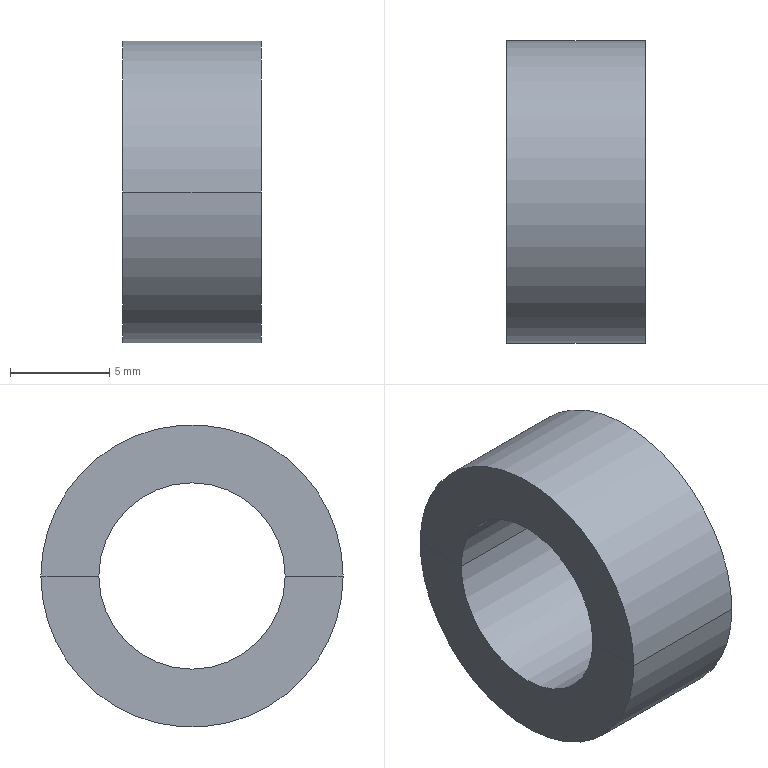Part | STEP file | BREP_9 | 1 solid | 8 faces | box 7 x 15.25 x 15.25 mm | volume 792.795 mm3 | cylinder 4 | plane 4 | commonest cylinder face diameters 9.4 x2 15.25 x2
STEP:
#1=CARTESIAN_POINT('',(0.,0.,0.));
#2=DIRECTION('',(0.,0.,1.));
#3=DIRECTION('',(1.,0.,0.));
#4=AXIS2_PLACEMENT_3D('',#1,#2,#3);
#5=CARTESIAN_POINT('',(63.38,-7.625,0.));
#6=VERTEX_POINT('',#5);
#7=CARTESIAN_POINT('',(70.38,-7.625,0.));
#8=VERTEX_POINT('',#7);
#9=CARTESIAN_POINT('',(63.38,-7.625,0.));
#10=DIRECTION('',(1.,0.,0.));
#11=VECTOR('',#10,1.);
#12=LINE('',#9,#11);
#13=CARTESIAN_POINT('',(66.88,0.,0.));
#14=DIRECTION('',(-1.,0.,0.));
#15=DIRECTION('',(0.,-1.,0.));
#16=AXIS2_PLACEMENT_3D('',#13,#14,#15);
#17=CYLINDRICAL_SURFACE('',#16,7.625);
#18=CARTESIAN_POINT('',(6.283,3.5));
#19=DIRECTION('',(0.,-1.));
#20=VECTOR('',#19,1.);
#21=LINE('',#18,#20);
#22=(GEOMETRIC_REPRESENTATION_CONTEXT(2)PARAMETRIC_REPRESENTATION_CONTEXT()REPRESENTATION_CONTEXT('',''));
#23=DEFINITIONAL_REPRESENTATION('',(#21),#22);
#24=PCURVE('',#17,#23);
#25=CARTESIAN_POINT('',(66.88,0.,0.));
#26=DIRECTION('',(-1.,0.,0.));
#27=DIRECTION('',(0.,1.,0.));
#28=AXIS2_PLACEMENT_3D('',#25,#26,#27);
#29=CYLINDRICAL_SURFACE('',#28,7.625);
#30=CARTESIAN_POINT('',(3.142,3.5));
#31=DIRECTION('',(0.,-1.));
#32=VECTOR('',#31,1.);
#33=LINE('',#30,#32);
#34=(GEOMETRIC_REPRESENTATION_CONTEXT(2)PARAMETRIC_REPRESENTATION_CONTEXT()REPRESENTATION_CONTEXT('',''));
#35=DEFINITIONAL_REPRESENTATION('',(#33),#34);
#36=PCURVE('',#29,#35);
#37=SURFACE_CURVE('',#12,(#24,#36),.PCURVE_S1.);
#38=EDGE_CURVE('',#6,#8,#37,.T.);
#39=ORIENTED_EDGE('',*,*,#38,.F.);
#40=CARTESIAN_POINT('',(63.38,7.625,0.));
#41=VERTEX_POINT('',#40);
#42=CARTESIAN_POINT('',(63.38,0.,0.));
#43=DIRECTION('',(-1.,0.,0.));
#44=DIRECTION('',(0.,1.,0.));
#45=AXIS2_PLACEMENT_3D('',#42,#43,#44);
#46=CIRCLE('',#45,7.625);
#47=CARTESIAN_POINT('',(3.142,3.5));
#48=DIRECTION('',(1.,0.));
#49=VECTOR('',#48,1.);
#50=LINE('',#47,#49);
#51=(GEOMETRIC_REPRESENTATION_CONTEXT(2)PARAMETRIC_REPRESENTATION_CONTEXT()REPRESENTATION_CONTEXT('',''));
#52=DEFINITIONAL_REPRESENTATION('',(#50),#51);
#53=PCURVE('',#17,#52);
#54=CARTESIAN_POINT('',(63.38,0.,-6.162));
#55=DIRECTION('',(1.,0.,0.));
#56=DIRECTION('',(0.,0.,1.));
#57=AXIS2_PLACEMENT_3D('',#54,#55,#56);
#58=PLANE('',#57);
#59=CARTESIAN_POINT('',(6.162,-7.625));
#60=CARTESIAN_POINT('',(-7.044,-7.625));
#61=CARTESIAN_POINT('',(-0.4409,3.812));
#62=CARTESIAN_POINT('',(6.162,15.25));
#63=CARTESIAN_POINT('',(12.766,3.812));
#64=CARTESIAN_POINT('',(19.369,-7.625));
#65=CARTESIAN_POINT('',(6.162,-7.625));
#66=(BOUNDED_CURVE()B_SPLINE_CURVE(2,(#59,#60,#61,#62,#63,#64,#65),.UNSPECIFIED.,.T.,.F.)B_SPLINE_CURVE_WITH_KNOTS((1,2,2,2,2,1),(-2.094,0.,2.094,4.189,6.283,8.378),.UNSPECIFIED.)CURVE()GEOMETRIC_REPRESENTATION_ITEM()RATIONAL_B_SPLINE_CURVE((1.,0.5,1.,0.5,1.,0.5,1.))REPRESENTATION_ITEM(''));
#67=(GEOMETRIC_REPRESENTATION_CONTEXT(2)PARAMETRIC_REPRESENTATION_CONTEXT()REPRESENTATION_CONTEXT('',''));
#68=DEFINITIONAL_REPRESENTATION('',(#66),#67);
#69=PCURVE('',#58,#68);
#70=SURFACE_CURVE('',#46,(#53,#69),.PCURVE_S1.);
#71=EDGE_CURVE('',#41,#6,#70,.T.);
#72=ORIENTED_EDGE('',*,*,#71,.F.);
#73=CARTESIAN_POINT('',(70.38,7.625,0.));
#74=VERTEX_POINT('',#73);
#75=CARTESIAN_POINT('',(63.38,7.625,0.));
#76=DIRECTION('',(1.,0.,0.));
#77=VECTOR('',#76,1.);
#78=LINE('',#75,#77);
#79=CARTESIAN_POINT('',(3.142,3.5));
#80=DIRECTION('',(0.,-1.));
#81=VECTOR('',#80,1.);
#82=LINE('',#79,#81);
#83=(GEOMETRIC_REPRESENTATION_CONTEXT(2)PARAMETRIC_REPRESENTATION_CONTEXT()REPRESENTATION_CONTEXT('',''));
#84=DEFINITIONAL_REPRESENTATION('',(#82),#83);
#85=PCURVE('',#17,#84);
#86=CARTESIAN_POINT('',(6.283,3.5));
#87=DIRECTION('',(0.,-1.));
#88=VECTOR('',#87,1.);
#89=LINE('',#86,#88);
#90=(GEOMETRIC_REPRESENTATION_CONTEXT(2)PARAMETRIC_REPRESENTATION_CONTEXT()REPRESENTATION_CONTEXT('',''));
#91=DEFINITIONAL_REPRESENTATION('',(#89),#90);
#92=PCURVE('',#29,#91);
#93=SURFACE_CURVE('',#78,(#85,#92),.PCURVE_S1.);
#94=EDGE_CURVE('',#41,#74,#93,.T.);
#95=ORIENTED_EDGE('',*,*,#94,.T.);
#96=CARTESIAN_POINT('',(70.38,0.,0.));
#97=DIRECTION('',(1.,0.,0.));
#98=DIRECTION('',(0.,-1.,0.));
#99=AXIS2_PLACEMENT_3D('',#96,#97,#98);
#100=CIRCLE('',#99,7.625);
#101=CARTESIAN_POINT('',(6.283,-3.5));
#102=DIRECTION('',(-1.,0.));
#103=VECTOR('',#102,1.);
#104=LINE('',#101,#103);
#105=(GEOMETRIC_REPRESENTATION_CONTEXT(2)PARAMETRIC_REPRESENTATION_CONTEXT()REPRESENTATION_CONTEXT('',''));
#106=DEFINITIONAL_REPRESENTATION('',(#104),#105);
#107=PCURVE('',#17,#106);
#108=CARTESIAN_POINT('',(70.38,0.,-6.162));
#109=DIRECTION('',(1.,0.,0.));
#110=DIRECTION('',(0.,0.,-1.));
#111=AXIS2_PLACEMENT_3D('',#108,#109,#110);
#112=PLANE('',#111);
#113=CARTESIAN_POINT('',(-6.162,0.));
#114=DIRECTION('',(0.,-1.));
#115=AXIS2_PLACEMENT_2D('',#113,#114);
#116=CIRCLE('',#115,7.625);
#117=(GEOMETRIC_REPRESENTATION_CONTEXT(2)PARAMETRIC_REPRESENTATION_CONTEXT()REPRESENTATION_CONTEXT('',''));
#118=DEFINITIONAL_REPRESENTATION('',(#116),#117);
#119=PCURVE('',#112,#118);
#120=SURFACE_CURVE('',#100,(#107,#119),.PCURVE_S1.);
#121=EDGE_CURVE('',#8,#74,#120,.T.);
#122=ORIENTED_EDGE('',*,*,#121,.F.);
#123=EDGE_LOOP('',(#39,#72,#95,#122));
#124=FACE_BOUND('',#123,.T.);
#125=ADVANCED_FACE('',(#124),#17,.T.);
#126=CARTESIAN_POINT('',(70.38,4.7,0.));
#127=VERTEX_POINT('',#126);
#128=CARTESIAN_POINT('',(70.38,-4.7,0.));
#129=VERTEX_POINT('',#128);
#130=CARTESIAN_POINT('',(70.38,0.,0.));
#131=DIRECTION('',(-1.,0.,0.));
#132=DIRECTION('',(0.,1.,0.));
#133=AXIS2_PLACEMENT_3D('',#130,#131,#132);
#134=CIRCLE('',#133,4.7);
#135=CARTESIAN_POINT('',(-6.162,4.7));
#136=CARTESIAN_POINT('',(1.978,4.7));
#137=CARTESIAN_POINT('',(-2.092,-2.35));
#138=CARTESIAN_POINT('',(-6.162,-9.4));
#139=CARTESIAN_POINT('',(-10.233,-2.35));
#140=CARTESIAN_POINT('',(-14.303,4.7));
#141=CARTESIAN_POINT('',(-6.162,4.7));
#142=(BOUNDED_CURVE()B_SPLINE_CURVE(2,(#135,#136,#137,#138,#139,#140,#141),.UNSPECIFIED.,.T.,.F.)B_SPLINE_CURVE_WITH_KNOTS((1,2,2,2,2,1),(-2.094,0.,2.094,4.189,6.283,8.378),.UNSPECIFIED.)CURVE()GEOMETRIC_REPRESENTATION_ITEM()RATIONAL_B_SPLINE_CURVE((1.,0.5,1.,0.5,1.,0.5,1.))REPRESENTATION_ITEM(''));
#143=(GEOMETRIC_REPRESENTATION_CONTEXT(2)PARAMETRIC_REPRESENTATION_CONTEXT()REPRESENTATION_CONTEXT('',''));
#144=DEFINITIONAL_REPRESENTATION('',(#142),#143);
#145=PCURVE('',#112,#144);
#146=CARTESIAN_POINT('',(66.88,0.,0.));
#147=DIRECTION('',(1.,0.,0.));
#148=DIRECTION('',(0.,1.,0.));
#149=AXIS2_PLACEMENT_3D('',#146,#147,#148);
#150=CYLINDRICAL_SURFACE('',#149,4.7);
#151=CARTESIAN_POINT('',(6.283,3.5));
#152=DIRECTION('',(-1.,0.));
#153=VECTOR('',#152,1.);
#154=LINE('',#151,#153);
#155=(GEOMETRIC_REPRESENTATION_CONTEXT(2)PARAMETRIC_REPRESENTATION_CONTEXT()REPRESENTATION_CONTEXT('',''));
#156=DEFINITIONAL_REPRESENTATION('',(#154),#155);
#157=PCURVE('',#150,#156);
#158=SURFACE_CURVE('',#134,(#145,#157),.PCURVE_S1.);
#159=EDGE_CURVE('',#127,#129,#158,.T.);
#160=ORIENTED_EDGE('',*,*,#159,.F.);
#161=CARTESIAN_POINT('',(70.38,7.625,0.));
#162=DIRECTION('',(0.,-1.,0.));
#163=VECTOR('',#162,1.);
#164=LINE('',#161,#163);
#165=CARTESIAN_POINT('',(-6.162,7.625));
#166=DIRECTION('',(0.,-1.));
#167=VECTOR('',#166,1.);
#168=LINE('',#165,#167);
#169=(GEOMETRIC_REPRESENTATION_CONTEXT(2)PARAMETRIC_REPRESENTATION_CONTEXT()REPRESENTATION_CONTEXT('',''));
#170=DEFINITIONAL_REPRESENTATION('',(#168),#169);
#171=PCURVE('',#112,#170);
#172=CARTESIAN_POINT('',(70.38,0.,6.162));
#173=DIRECTION('',(1.,0.,0.));
#174=DIRECTION('',(0.,0.,1.));
#175=AXIS2_PLACEMENT_3D('',#172,#173,#174);
#176=PLANE('',#175);
#177=CARTESIAN_POINT('',(-6.162,-7.625));
#178=DIRECTION('',(0.,1.));
#179=VECTOR('',#178,1.);
#180=LINE('',#177,#179);
#181=(GEOMETRIC_REPRESENTATION_CONTEXT(2)PARAMETRIC_REPRESENTATION_CONTEXT()REPRESENTATION_CONTEXT('',''));
#182=DEFINITIONAL_REPRESENTATION('',(#180),#181);
#183=PCURVE('',#176,#182);
#184=SURFACE_CURVE('',#164,(#171,#183),.PCURVE_S1.);
#185=EDGE_CURVE('',#74,#127,#184,.T.);
#186=ORIENTED_EDGE('',*,*,#185,.F.);
#187=ORIENTED_EDGE('',*,*,#121,.F.);
#188=CARTESIAN_POINT('',(70.38,-7.625,0.));
#189=DIRECTION('',(0.,1.,0.));
#190=VECTOR('',#189,1.);
#191=LINE('',#188,#190);
#192=CARTESIAN_POINT('',(-6.162,-7.625));
#193=DIRECTION('',(0.,1.));
#194=VECTOR('',#193,1.);
#195=LINE('',#192,#194);
#196=(GEOMETRIC_REPRESENTATION_CONTEXT(2)PARAMETRIC_REPRESENTATION_CONTEXT()REPRESENTATION_CONTEXT('',''));
#197=DEFINITIONAL_REPRESENTATION('',(#195),#196);
#198=PCURVE('',#112,#197);
#199=CARTESIAN_POINT('',(-6.162,7.625));
#200=DIRECTION('',(0.,-1.));
#201=VECTOR('',#200,1.);
#202=LINE('',#199,#201);
#203=(GEOMETRIC_REPRESENTATION_CONTEXT(2)PARAMETRIC_REPRESENTATION_CONTEXT()REPRESENTATION_CONTEXT('',''));
#204=DEFINITIONAL_REPRESENTATION('',(#202),#203);
#205=PCURVE('',#176,#204);
#206=SURFACE_CURVE('',#191,(#198,#205),.PCURVE_S1.);
#207=EDGE_CURVE('',#8,#129,#206,.T.);
#208=ORIENTED_EDGE('',*,*,#207,.T.);
#209=EDGE_LOOP('',(#160,#186,#187,#208));
#210=FACE_BOUND('',#209,.F.);
#211=ADVANCED_FACE('',(#210),#112,.T.);
#212=CARTESIAN_POINT('',(63.38,-4.7,0.));
#213=VERTEX_POINT('',#212);
#214=CARTESIAN_POINT('',(70.38,-4.7,0.));
#215=DIRECTION('',(-1.,0.,0.));
#216=VECTOR('',#215,1.);
#217=LINE('',#214,#216);
#218=CARTESIAN_POINT('',(3.142,3.5));
#219=DIRECTION('',(0.,-1.));
#220=VECTOR('',#219,1.);
#221=LINE('',#218,#220);
#222=(GEOMETRIC_REPRESENTATION_CONTEXT(2)PARAMETRIC_REPRESENTATION_CONTEXT()REPRESENTATION_CONTEXT('',''));
#223=DEFINITIONAL_REPRESENTATION('',(#221),#222);
#224=PCURVE('',#150,#223);
#225=CARTESIAN_POINT('',(66.88,0.,0.));
#226=DIRECTION('',(1.,0.,0.));
#227=DIRECTION('',(0.,-1.,0.));
#228=AXIS2_PLACEMENT_3D('',#225,#226,#227);
#229=CYLINDRICAL_SURFACE('',#228,4.7);
#230=CARTESIAN_POINT('',(6.283,3.5));
#231=DIRECTION('',(0.,-1.));
#232=VECTOR('',#231,1.);
#233=LINE('',#230,#232);
#234=(GEOMETRIC_REPRESENTATION_CONTEXT(2)PARAMETRIC_REPRESENTATION_CONTEXT()REPRESENTATION_CONTEXT('',''));
#235=DEFINITIONAL_REPRESENTATION('',(#233),#234);
#236=PCURVE('',#229,#235);
#237=SURFACE_CURVE('',#217,(#224,#236),.PCURVE_S1.);
#238=EDGE_CURVE('',#129,#213,#237,.T.);
#239=ORIENTED_EDGE('',*,*,#238,.T.);
#240=CARTESIAN_POINT('',(63.38,4.7,0.));
#241=VERTEX_POINT('',#240);
#242=CARTESIAN_POINT('',(63.38,0.,0.));
#243=DIRECTION('',(1.,0.,0.));
#244=DIRECTION('',(0.,-1.,0.));
#245=AXIS2_PLACEMENT_3D('',#242,#243,#244);
#246=CIRCLE('',#245,4.7);
#247=CARTESIAN_POINT('',(3.142,-3.5));
#248=DIRECTION('',(1.,0.));
#249=VECTOR('',#248,1.);
#250=LINE('',#247,#249);
#251=(GEOMETRIC_REPRESENTATION_CONTEXT(2)PARAMETRIC_REPRESENTATION_CONTEXT()REPRESENTATION_CONTEXT('',''));
#252=DEFINITIONAL_REPRESENTATION('',(#250),#251);
#253=PCURVE('',#150,#252);
#254=CARTESIAN_POINT('',(6.162,0.));
#255=DIRECTION('',(0.,1.));
#256=AXIS2_PLACEMENT_2D('',#254,#255);
#257=CIRCLE('',#256,4.7);
#258=(GEOMETRIC_REPRESENTATION_CONTEXT(2)PARAMETRIC_REPRESENTATION_CONTEXT()REPRESENTATION_CONTEXT('',''));
#259=DEFINITIONAL_REPRESENTATION('',(#257),#258);
#260=PCURVE('',#58,#259);
#261=SURFACE_CURVE('',#246,(#253,#260),.PCURVE_S1.);
#262=EDGE_CURVE('',#213,#241,#261,.T.);
#263=ORIENTED_EDGE('',*,*,#262,.T.);
#264=CARTESIAN_POINT('',(70.38,4.7,0.));
#265=DIRECTION('',(-1.,0.,0.));
#266=VECTOR('',#265,1.);
#267=LINE('',#264,#266);
#268=CARTESIAN_POINT('',(6.283,3.5));
#269=DIRECTION('',(0.,-1.));
#270=VECTOR('',#269,1.);
#271=LINE('',#268,#270);
#272=(GEOMETRIC_REPRESENTATION_CONTEXT(2)PARAMETRIC_REPRESENTATION_CONTEXT()REPRESENTATION_CONTEXT('',''));
#273=DEFINITIONAL_REPRESENTATION('',(#271),#272);
#274=PCURVE('',#150,#273);
#275=CARTESIAN_POINT('',(3.142,3.5));
#276=DIRECTION('',(0.,-1.));
#277=VECTOR('',#276,1.);
#278=LINE('',#275,#277);
#279=(GEOMETRIC_REPRESENTATION_CONTEXT(2)PARAMETRIC_REPRESENTATION_CONTEXT()REPRESENTATION_CONTEXT('',''));
#280=DEFINITIONAL_REPRESENTATION('',(#278),#279);
#281=PCURVE('',#229,#280);
#282=SURFACE_CURVE('',#267,(#274,#281),.PCURVE_S1.);
#283=EDGE_CURVE('',#127,#241,#282,.T.);
#284=ORIENTED_EDGE('',*,*,#283,.F.);
#285=ORIENTED_EDGE('',*,*,#159,.T.);
#286=EDGE_LOOP('',(#239,#263,#284,#285));
#287=FACE_BOUND('',#286,.F.);
#288=ADVANCED_FACE('',(#287),#150,.F.);
#289=CARTESIAN_POINT('',(63.38,0.,0.));
#290=DIRECTION('',(1.,0.,0.));
#291=DIRECTION('',(0.,1.,0.));
#292=AXIS2_PLACEMENT_3D('',#289,#290,#291);
#293=CIRCLE('',#292,4.7);
#294=CARTESIAN_POINT('',(3.142,-3.5));
#295=DIRECTION('',(1.,0.));
#296=VECTOR('',#295,1.);
#297=LINE('',#294,#296);
#298=(GEOMETRIC_REPRESENTATION_CONTEXT(2)PARAMETRIC_REPRESENTATION_CONTEXT()REPRESENTATION_CONTEXT('',''));
#299=DEFINITIONAL_REPRESENTATION('',(#297),#298);
#300=PCURVE('',#229,#299);
#301=CARTESIAN_POINT('',(63.38,0.,6.162));
#302=DIRECTION('',(1.,0.,0.));
#303=DIRECTION('',(0.,0.,-1.));
#304=AXIS2_PLACEMENT_3D('',#301,#302,#303);
#305=PLANE('',#304);
#306=CARTESIAN_POINT('',(6.162,0.));
#307=DIRECTION('',(0.,1.));
#308=AXIS2_PLACEMENT_2D('',#306,#307);
#309=CIRCLE('',#308,4.7);
#310=(GEOMETRIC_REPRESENTATION_CONTEXT(2)PARAMETRIC_REPRESENTATION_CONTEXT()REPRESENTATION_CONTEXT('',''));
#311=DEFINITIONAL_REPRESENTATION('',(#309),#310);
#312=PCURVE('',#305,#311);
#313=SURFACE_CURVE('',#293,(#300,#312),.PCURVE_S1.);
#314=EDGE_CURVE('',#241,#213,#313,.T.);
#315=ORIENTED_EDGE('',*,*,#314,.T.);
#316=ORIENTED_EDGE('',*,*,#238,.F.);
#317=CARTESIAN_POINT('',(70.38,0.,0.));
#318=DIRECTION('',(-1.,0.,0.));
#319=DIRECTION('',(0.,-1.,0.));
#320=AXIS2_PLACEMENT_3D('',#317,#318,#319);
#321=CIRCLE('',#320,4.7);
#322=CARTESIAN_POINT('',(6.283,3.5));
#323=DIRECTION('',(-1.,0.));
#324=VECTOR('',#323,1.);
#325=LINE('',#322,#324);
#326=(GEOMETRIC_REPRESENTATION_CONTEXT(2)PARAMETRIC_REPRESENTATION_CONTEXT()REPRESENTATION_CONTEXT('',''));
#327=DEFINITIONAL_REPRESENTATION('',(#325),#326);
#328=PCURVE('',#229,#327);
#329=CARTESIAN_POINT('',(-6.162,4.7));
#330=CARTESIAN_POINT('',(1.978,4.7));
#331=CARTESIAN_POINT('',(-2.092,-2.35));
#332=CARTESIAN_POINT('',(-6.162,-9.4));
#333=CARTESIAN_POINT('',(-10.233,-2.35));
#334=CARTESIAN_POINT('',(-14.303,4.7));
#335=CARTESIAN_POINT('',(-6.162,4.7));
#336=(BOUNDED_CURVE()B_SPLINE_CURVE(2,(#329,#330,#331,#332,#333,#334,#335),.UNSPECIFIED.,.T.,.F.)B_SPLINE_CURVE_WITH_KNOTS((1,2,2,2,2,1),(-2.094,0.,2.094,4.189,6.283,8.378),.UNSPECIFIED.)CURVE()GEOMETRIC_REPRESENTATION_ITEM()RATIONAL_B_SPLINE_CURVE((1.,0.5,1.,0.5,1.,0.5,1.))REPRESENTATION_ITEM(''));
#337=(GEOMETRIC_REPRESENTATION_CONTEXT(2)PARAMETRIC_REPRESENTATION_CONTEXT()REPRESENTATION_CONTEXT('',''));
#338=DEFINITIONAL_REPRESENTATION('',(#336),#337);
#339=PCURVE('',#176,#338);
#340=SURFACE_CURVE('',#321,(#328,#339),.PCURVE_S1.);
#341=EDGE_CURVE('',#129,#127,#340,.T.);
#342=ORIENTED_EDGE('',*,*,#341,.T.);
#343=ORIENTED_EDGE('',*,*,#283,.T.);
#344=EDGE_LOOP('',(#315,#316,#342,#343));
#345=FACE_BOUND('',#344,.F.);
#346=ADVANCED_FACE('',(#345),#229,.F.);
#347=CARTESIAN_POINT('',(63.38,4.7,0.));
#348=DIRECTION('',(0.,1.,0.));
#349=VECTOR('',#348,1.);
#350=LINE('',#347,#349);
#351=CARTESIAN_POINT('',(6.162,4.7));
#352=DIRECTION('',(0.,1.));
#353=VECTOR('',#352,1.);
#354=LINE('',#351,#353);
#355=(GEOMETRIC_REPRESENTATION_CONTEXT(2)PARAMETRIC_REPRESENTATION_CONTEXT()REPRESENTATION_CONTEXT('',''));
#356=DEFINITIONAL_REPRESENTATION('',(#354),#355);
#357=PCURVE('',#305,#356);
#358=CARTESIAN_POINT('',(6.162,-4.7));
#359=DIRECTION('',(0.,-1.));
#360=VECTOR('',#359,1.);
#361=LINE('',#358,#360);
#362=(GEOMETRIC_REPRESENTATION_CONTEXT(2)PARAMETRIC_REPRESENTATION_CONTEXT()REPRESENTATION_CONTEXT('',''));
#363=DEFINITIONAL_REPRESENTATION('',(#361),#362);
#364=PCURVE('',#58,#363);
#365=SURFACE_CURVE('',#350,(#357,#364),.PCURVE_S1.);
#366=EDGE_CURVE('',#241,#41,#365,.T.);
#367=ORIENTED_EDGE('',*,*,#366,.T.);
#368=CARTESIAN_POINT('',(63.38,0.,0.));
#369=DIRECTION('',(-1.,0.,0.));
#370=DIRECTION('',(0.,-1.,0.));
#371=AXIS2_PLACEMENT_3D('',#368,#369,#370);
#372=CIRCLE('',#371,7.625);
#373=CARTESIAN_POINT('',(6.162,-7.625));
#374=CARTESIAN_POINT('',(-7.044,-7.625));
#375=CARTESIAN_POINT('',(-0.4409,3.812));
#376=CARTESIAN_POINT('',(6.162,15.25));
#377=CARTESIAN_POINT('',(12.766,3.812));
#378=CARTESIAN_POINT('',(19.369,-7.625));
#379=CARTESIAN_POINT('',(6.162,-7.625));
#380=(BOUNDED_CURVE()B_SPLINE_CURVE(2,(#373,#374,#375,#376,#377,#378,#379),.UNSPECIFIED.,.T.,.F.)B_SPLINE_CURVE_WITH_KNOTS((1,2,2,2,2,1),(-2.094,0.,2.094,4.189,6.283,8.378),.UNSPECIFIED.)CURVE()GEOMETRIC_REPRESENTATION_ITEM()RATIONAL_B_SPLINE_CURVE((1.,0.5,1.,0.5,1.,0.5,1.))REPRESENTATION_ITEM(''));
#381=(GEOMETRIC_REPRESENTATION_CONTEXT(2)PARAMETRIC_REPRESENTATION_CONTEXT()REPRESENTATION_CONTEXT('',''));
#382=DEFINITIONAL_REPRESENTATION('',(#380),#381);
#383=PCURVE('',#305,#382);
#384=CARTESIAN_POINT('',(3.142,3.5));
#385=DIRECTION('',(1.,0.));
#386=VECTOR('',#385,1.);
#387=LINE('',#384,#386);
#388=(GEOMETRIC_REPRESENTATION_CONTEXT(2)PARAMETRIC_REPRESENTATION_CONTEXT()REPRESENTATION_CONTEXT('',''));
#389=DEFINITIONAL_REPRESENTATION('',(#387),#388);
#390=PCURVE('',#29,#389);
#391=SURFACE_CURVE('',#372,(#383,#390),.PCURVE_S1.);
#392=EDGE_CURVE('',#6,#41,#391,.T.);
#393=ORIENTED_EDGE('',*,*,#392,.F.);
#394=CARTESIAN_POINT('',(63.38,-4.7,0.));
#395=DIRECTION('',(0.,-1.,0.));
#396=VECTOR('',#395,1.);
#397=LINE('',#394,#396);
#398=CARTESIAN_POINT('',(6.162,-4.7));
#399=DIRECTION('',(0.,-1.));
#400=VECTOR('',#399,1.);
#401=LINE('',#398,#400);
#402=(GEOMETRIC_REPRESENTATION_CONTEXT(2)PARAMETRIC_REPRESENTATION_CONTEXT()REPRESENTATION_CONTEXT('',''));
#403=DEFINITIONAL_REPRESENTATION('',(#401),#402);
#404=PCURVE('',#305,#403);
#405=CARTESIAN_POINT('',(6.162,4.7));
#406=DIRECTION('',(0.,1.));
#407=VECTOR('',#406,1.);
#408=LINE('',#405,#407);
#409=(GEOMETRIC_REPRESENTATION_CONTEXT(2)PARAMETRIC_REPRESENTATION_CONTEXT()REPRESENTATION_CONTEXT('',''));
#410=DEFINITIONAL_REPRESENTATION('',(#408),#409);
#411=PCURVE('',#58,#410);
#412=SURFACE_CURVE('',#397,(#404,#411),.PCURVE_S1.);
#413=EDGE_CURVE('',#213,#6,#412,.T.);
#414=ORIENTED_EDGE('',*,*,#413,.F.);
#415=ORIENTED_EDGE('',*,*,#314,.F.);
#416=EDGE_LOOP('',(#367,#393,#414,#415));
#417=FACE_BOUND('',#416,.F.);
#418=ADVANCED_FACE('',(#417),#305,.F.);
#419=ORIENTED_EDGE('',*,*,#71,.F.);
#420=ORIENTED_EDGE('',*,*,#366,.F.);
#421=ORIENTED_EDGE('',*,*,#262,.F.);
#422=ORIENTED_EDGE('',*,*,#413,.T.);
#423=EDGE_LOOP('',(#419,#420,#421,#422));
#424=FACE_BOUND('',#423,.F.);
#425=ADVANCED_FACE('',(#424),#58,.F.);
#426=ORIENTED_EDGE('',*,*,#392,.F.);
#427=ORIENTED_EDGE('',*,*,#38,.T.);
#428=CARTESIAN_POINT('',(70.38,0.,0.));
#429=DIRECTION('',(1.,0.,0.));
#430=DIRECTION('',(0.,1.,0.));
#431=AXIS2_PLACEMENT_3D('',#428,#429,#430);
#432=CIRCLE('',#431,7.625);
#433=CARTESIAN_POINT('',(6.283,-3.5));
#434=DIRECTION('',(-1.,0.));
#435=VECTOR('',#434,1.);
#436=LINE('',#433,#435);
#437=(GEOMETRIC_REPRESENTATION_CONTEXT(2)PARAMETRIC_REPRESENTATION_CONTEXT()REPRESENTATION_CONTEXT('',''));
#438=DEFINITIONAL_REPRESENTATION('',(#436),#437);
#439=PCURVE('',#29,#438);
#440=CARTESIAN_POINT('',(-6.162,0.));
#441=DIRECTION('',(0.,-1.));
#442=AXIS2_PLACEMENT_2D('',#440,#441);
#443=CIRCLE('',#442,7.625);
#444=(GEOMETRIC_REPRESENTATION_CONTEXT(2)PARAMETRIC_REPRESENTATION_CONTEXT()REPRESENTATION_CONTEXT('',''));
#445=DEFINITIONAL_REPRESENTATION('',(#443),#444);
#446=PCURVE('',#176,#445);
#447=SURFACE_CURVE('',#432,(#439,#446),.PCURVE_S1.);
#448=EDGE_CURVE('',#74,#8,#447,.T.);
#449=ORIENTED_EDGE('',*,*,#448,.F.);
#450=ORIENTED_EDGE('',*,*,#94,.F.);
#451=EDGE_LOOP('',(#426,#427,#449,#450));
#452=FACE_BOUND('',#451,.T.);
#453=ADVANCED_FACE('',(#452),#29,.T.);
#454=ORIENTED_EDGE('',*,*,#185,.T.);
#455=ORIENTED_EDGE('',*,*,#341,.F.);
#456=ORIENTED_EDGE('',*,*,#207,.F.);
#457=ORIENTED_EDGE('',*,*,#448,.F.);
#458=EDGE_LOOP('',(#454,#455,#456,#457));
#459=FACE_BOUND('',#458,.F.);
#460=ADVANCED_FACE('',(#459),#176,.T.);
#461=CLOSED_SHELL('',(#125,#211,#288,#346,#418,#425,#453,#460));
#462=MANIFOLD_SOLID_BREP('',#461);
#463=(LENGTH_UNIT()NAMED_UNIT(*)SI_UNIT(.MILLI.,.METRE.));
#464=UNCERTAINTY_MEASURE_WITH_UNIT(LENGTH_MEASURE(0.0000001),#463,'','');
#465=(NAMED_UNIT(*)PLANE_ANGLE_UNIT()SI_UNIT($,.RADIAN.));
#466=(NAMED_UNIT(*)SI_UNIT($,.STERADIAN.)SOLID_ANGLE_UNIT());
#467=(GEOMETRIC_REPRESENTATION_CONTEXT(3)GLOBAL_UNCERTAINTY_ASSIGNED_CONTEXT((#464))GLOBAL_UNIT_ASSIGNED_CONTEXT((#463,#465,#466))REPRESENTATION_CONTEXT('',''));
#468=ADVANCED_BREP_SHAPE_REPRESENTATION('',(#4,#462),#467);